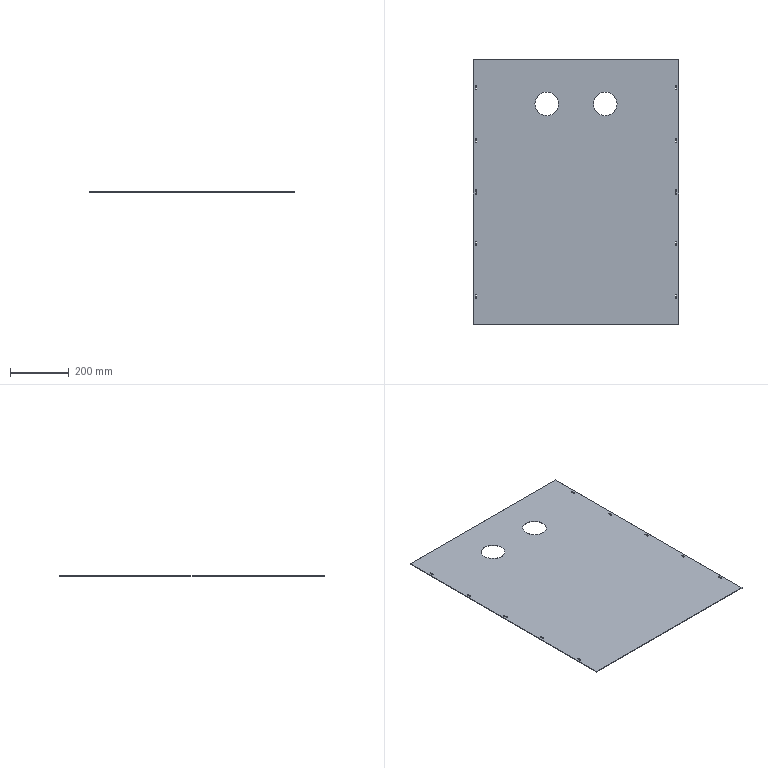Part | SolidWorks | features ICE 2, Extrusion 1 | 1 solid | 50 faces | box 700 x 900 x 2 mm | volume 1238676 mm3 | plane 26 | cylinder 24 | commonest cylinder face diameters 4.5 x20 80 x4